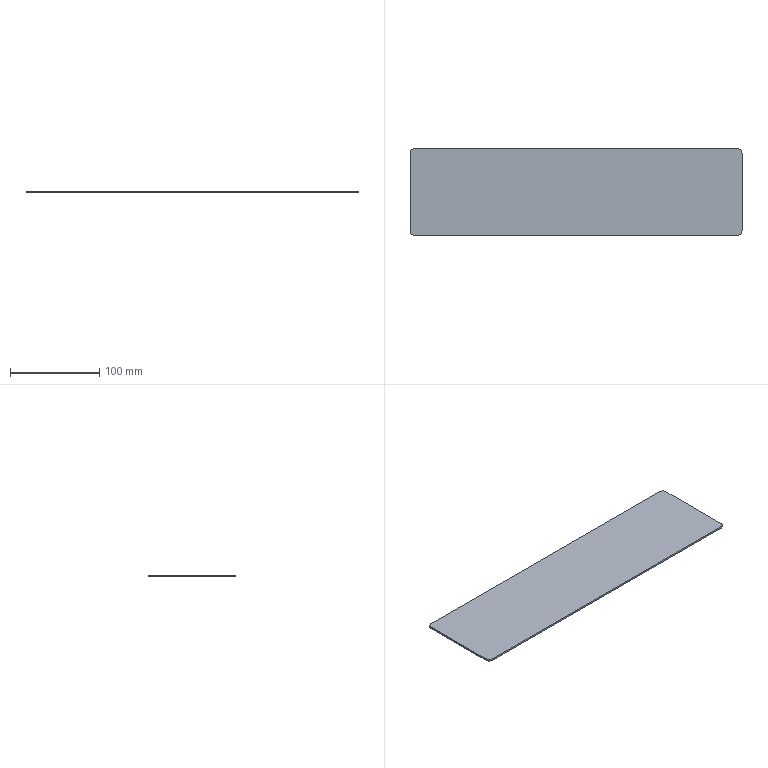Part | SolidWorks | features FlatPattern 1, SMBaseFlange 1, SheetMetal 1 | 1 solid | 10 faces | box 372 x 97 x 2 mm | volume 72125 mm3 | plane 6 | cylinder 4 | commonest cylinder face diameters 10 x4
STEP:
#1=CARTESIAN_POINT('',(0.,-92.,0.));
#2=VERTEX_POINT('',#1);
#3=CARTESIAN_POINT('',(5.,-97.,0.));
#4=VERTEX_POINT('',#3);
#5=CARTESIAN_POINT('',(5.,-92.,0.));
#6=DIRECTION('',(0.,0.,1.));
#7=DIRECTION('',(1.,0.,0.));
#8=AXIS2_PLACEMENT_3D('',#5,#6,#7);
#9=CIRCLE('',#8,5.);
#10=EDGE_CURVE('',#2,#4,#9,.T.);
#11=ORIENTED_EDGE('',*,*,#10,.F.);
#12=CARTESIAN_POINT('',(0.,-92.,-2.));
#13=VERTEX_POINT('',#12);
#14=CARTESIAN_POINT('',(0.,-92.,-2.));
#15=DIRECTION('',(0.,0.,1.));
#16=VECTOR('',#15,1000.);
#17=LINE('',#14,#16);
#18=EDGE_CURVE('',#13,#2,#17,.T.);
#19=ORIENTED_EDGE('',*,*,#18,.F.);
#20=CARTESIAN_POINT('',(5.,-97.,-2.));
#21=VERTEX_POINT('',#20);
#22=CARTESIAN_POINT('',(5.,-92.,-2.));
#23=DIRECTION('',(0.,0.,1.));
#24=DIRECTION('',(1.,0.,0.));
#25=AXIS2_PLACEMENT_3D('',#22,#23,#24);
#26=CIRCLE('',#25,5.);
#27=EDGE_CURVE('',#13,#21,#26,.T.);
#28=ORIENTED_EDGE('',*,*,#27,.T.);
#29=CARTESIAN_POINT('',(5.,-97.,-2.));
#30=DIRECTION('',(0.,0.,1.));
#31=VECTOR('',#30,1000.);
#32=LINE('',#29,#31);
#33=EDGE_CURVE('',#21,#4,#32,.T.);
#34=ORIENTED_EDGE('',*,*,#33,.T.);
#35=EDGE_LOOP('',(#11,#19,#28,#34));
#36=FACE_OUTER_BOUND('',#35,.T.);
#37=CARTESIAN_POINT('',(5.,-92.,-2.));
#38=DIRECTION('',(0.,0.,1.));
#39=DIRECTION('',(1.,0.,0.));
#40=AXIS2_PLACEMENT_3D('',#37,#38,#39);
#41=CYLINDRICAL_SURFACE('',#40,5.);
#42=ADVANCED_FACE('',(#36),#41,.T.);
#43=CARTESIAN_POINT('',(0.,-5.,0.));
#44=VERTEX_POINT('',#43);
#45=CARTESIAN_POINT('',(0.,-5.,0.));
#46=DIRECTION('',(0.,-1.,0.));
#47=VECTOR('',#46,1000.);
#48=LINE('',#45,#47);
#49=EDGE_CURVE('',#44,#2,#48,.T.);
#50=ORIENTED_EDGE('',*,*,#49,.F.);
#51=CARTESIAN_POINT('',(0.,-5.,-2.));
#52=VERTEX_POINT('',#51);
#53=CARTESIAN_POINT('',(0.,-5.,-2.));
#54=DIRECTION('',(0.,0.,1.));
#55=VECTOR('',#54,1000.);
#56=LINE('',#53,#55);
#57=EDGE_CURVE('',#52,#44,#56,.T.);
#58=ORIENTED_EDGE('',*,*,#57,.F.);
#59=CARTESIAN_POINT('',(0.,-5.,-2.));
#60=DIRECTION('',(0.,-1.,0.));
#61=VECTOR('',#60,1000.);
#62=LINE('',#59,#61);
#63=EDGE_CURVE('',#52,#13,#62,.T.);
#64=ORIENTED_EDGE('',*,*,#63,.T.);
#65=ORIENTED_EDGE('',*,*,#18,.T.);
#66=EDGE_LOOP('',(#50,#58,#64,#65));
#67=FACE_OUTER_BOUND('',#66,.T.);
#68=CARTESIAN_POINT('',(0.,-5.,-2.));
#69=DIRECTION('',(-1.,0.,0.));
#70=DIRECTION('',(0.,-1.,0.));
#71=AXIS2_PLACEMENT_3D('',#68,#69,#70);
#72=PLANE('',#71);
#73=ADVANCED_FACE('',(#67),#72,.T.);
#74=CARTESIAN_POINT('',(5.,0.,0.));
#75=VERTEX_POINT('',#74);
#76=CARTESIAN_POINT('',(5.,-5.,0.));
#77=DIRECTION('',(0.,0.,1.));
#78=DIRECTION('',(1.,0.,0.));
#79=AXIS2_PLACEMENT_3D('',#76,#77,#78);
#80=CIRCLE('',#79,5.);
#81=EDGE_CURVE('',#75,#44,#80,.T.);
#82=ORIENTED_EDGE('',*,*,#81,.F.);
#83=CARTESIAN_POINT('',(5.,0.,-2.));
#84=VERTEX_POINT('',#83);
#85=CARTESIAN_POINT('',(5.,0.,-2.));
#86=DIRECTION('',(0.,0.,1.));
#87=VECTOR('',#86,1000.);
#88=LINE('',#85,#87);
#89=EDGE_CURVE('',#84,#75,#88,.T.);
#90=ORIENTED_EDGE('',*,*,#89,.F.);
#91=CARTESIAN_POINT('',(5.,-5.,-2.));
#92=DIRECTION('',(0.,0.,1.));
#93=DIRECTION('',(1.,0.,0.));
#94=AXIS2_PLACEMENT_3D('',#91,#92,#93);
#95=CIRCLE('',#94,5.);
#96=EDGE_CURVE('',#84,#52,#95,.T.);
#97=ORIENTED_EDGE('',*,*,#96,.T.);
#98=ORIENTED_EDGE('',*,*,#57,.T.);
#99=EDGE_LOOP('',(#82,#90,#97,#98));
#100=FACE_OUTER_BOUND('',#99,.T.);
#101=CARTESIAN_POINT('',(5.,-5.,-2.));
#102=DIRECTION('',(0.,0.,1.));
#103=DIRECTION('',(1.,0.,0.));
#104=AXIS2_PLACEMENT_3D('',#101,#102,#103);
#105=CYLINDRICAL_SURFACE('',#104,5.);
#106=ADVANCED_FACE('',(#100),#105,.T.);
#107=CARTESIAN_POINT('',(367.,0.,0.));
#108=VERTEX_POINT('',#107);
#109=CARTESIAN_POINT('',(5.,0.,0.));
#110=DIRECTION('',(-1.,0.,0.));
#111=VECTOR('',#110,1000.);
#112=LINE('',#109,#111);
#113=EDGE_CURVE('',#108,#75,#112,.T.);
#114=ORIENTED_EDGE('',*,*,#113,.F.);
#115=CARTESIAN_POINT('',(367.,0.,-2.));
#116=VERTEX_POINT('',#115);
#117=CARTESIAN_POINT('',(367.,0.,-2.));
#118=DIRECTION('',(0.,0.,1.));
#119=VECTOR('',#118,1000.);
#120=LINE('',#117,#119);
#121=EDGE_CURVE('',#116,#108,#120,.T.);
#122=ORIENTED_EDGE('',*,*,#121,.F.);
#123=CARTESIAN_POINT('',(5.,0.,-2.));
#124=DIRECTION('',(-1.,0.,0.));
#125=VECTOR('',#124,1000.);
#126=LINE('',#123,#125);
#127=EDGE_CURVE('',#116,#84,#126,.T.);
#128=ORIENTED_EDGE('',*,*,#127,.T.);
#129=ORIENTED_EDGE('',*,*,#89,.T.);
#130=EDGE_LOOP('',(#114,#122,#128,#129));
#131=FACE_OUTER_BOUND('',#130,.T.);
#132=CARTESIAN_POINT('',(5.,0.,-2.));
#133=DIRECTION('',(0.,1.,0.));
#134=DIRECTION('',(0.,0.,1.));
#135=AXIS2_PLACEMENT_3D('',#132,#133,#134);
#136=PLANE('',#135);
#137=ADVANCED_FACE('',(#131),#136,.T.);
#138=CARTESIAN_POINT('',(372.,-5.,0.));
#139=VERTEX_POINT('',#138);
#140=CARTESIAN_POINT('',(367.,-5.,0.));
#141=DIRECTION('',(0.,0.,1.));
#142=DIRECTION('',(-1.,0.,0.));
#143=AXIS2_PLACEMENT_3D('',#140,#141,#142);
#144=CIRCLE('',#143,5.);
#145=EDGE_CURVE('',#139,#108,#144,.T.);
#146=ORIENTED_EDGE('',*,*,#145,.F.);
#147=CARTESIAN_POINT('',(372.,-5.,-2.));
#148=VERTEX_POINT('',#147);
#149=CARTESIAN_POINT('',(372.,-5.,-2.));
#150=DIRECTION('',(0.,0.,1.));
#151=VECTOR('',#150,1000.);
#152=LINE('',#149,#151);
#153=EDGE_CURVE('',#148,#139,#152,.T.);
#154=ORIENTED_EDGE('',*,*,#153,.F.);
#155=CARTESIAN_POINT('',(367.,-5.,-2.));
#156=DIRECTION('',(0.,0.,1.));
#157=DIRECTION('',(-1.,0.,0.));
#158=AXIS2_PLACEMENT_3D('',#155,#156,#157);
#159=CIRCLE('',#158,5.);
#160=EDGE_CURVE('',#148,#116,#159,.T.);
#161=ORIENTED_EDGE('',*,*,#160,.T.);
#162=ORIENTED_EDGE('',*,*,#121,.T.);
#163=EDGE_LOOP('',(#146,#154,#161,#162));
#164=FACE_OUTER_BOUND('',#163,.T.);
#165=CARTESIAN_POINT('',(367.,-5.,-2.));
#166=DIRECTION('',(0.,0.,1.));
#167=DIRECTION('',(1.,0.,0.));
#168=AXIS2_PLACEMENT_3D('',#165,#166,#167);
#169=CYLINDRICAL_SURFACE('',#168,5.);
#170=ADVANCED_FACE('',(#164),#169,.T.);
#171=CARTESIAN_POINT('',(372.,-92.,0.));
#172=VERTEX_POINT('',#171);
#173=CARTESIAN_POINT('',(372.,-5.,0.));
#174=DIRECTION('',(0.,1.,0.));
#175=VECTOR('',#174,1000.);
#176=LINE('',#173,#175);
#177=EDGE_CURVE('',#172,#139,#176,.T.);
#178=ORIENTED_EDGE('',*,*,#177,.F.);
#179=CARTESIAN_POINT('',(372.,-92.,-2.));
#180=VERTEX_POINT('',#179);
#181=CARTESIAN_POINT('',(372.,-92.,-2.));
#182=DIRECTION('',(0.,0.,1.));
#183=VECTOR('',#182,1000.);
#184=LINE('',#181,#183);
#185=EDGE_CURVE('',#180,#172,#184,.T.);
#186=ORIENTED_EDGE('',*,*,#185,.F.);
#187=CARTESIAN_POINT('',(372.,-5.,-2.));
#188=DIRECTION('',(0.,1.,0.));
#189=VECTOR('',#188,1000.);
#190=LINE('',#187,#189);
#191=EDGE_CURVE('',#180,#148,#190,.T.);
#192=ORIENTED_EDGE('',*,*,#191,.T.);
#193=ORIENTED_EDGE('',*,*,#153,.T.);
#194=EDGE_LOOP('',(#178,#186,#192,#193));
#195=FACE_OUTER_BOUND('',#194,.T.);
#196=CARTESIAN_POINT('',(372.,-5.,-2.));
#197=DIRECTION('',(1.,0.,0.));
#198=DIRECTION('',(0.,0.,-1.));
#199=AXIS2_PLACEMENT_3D('',#196,#197,#198);
#200=PLANE('',#199);
#201=ADVANCED_FACE('',(#195),#200,.T.);
#202=CARTESIAN_POINT('',(367.,-97.,0.));
#203=VERTEX_POINT('',#202);
#204=CARTESIAN_POINT('',(367.,-92.,0.));
#205=DIRECTION('',(0.,0.,1.));
#206=DIRECTION('',(1.,0.,0.));
#207=AXIS2_PLACEMENT_3D('',#204,#205,#206);
#208=CIRCLE('',#207,5.);
#209=EDGE_CURVE('',#203,#172,#208,.T.);
#210=ORIENTED_EDGE('',*,*,#209,.F.);
#211=CARTESIAN_POINT('',(367.,-97.,-2.));
#212=VERTEX_POINT('',#211);
#213=CARTESIAN_POINT('',(367.,-97.,-2.));
#214=DIRECTION('',(0.,0.,1.));
#215=VECTOR('',#214,1000.);
#216=LINE('',#213,#215);
#217=EDGE_CURVE('',#212,#203,#216,.T.);
#218=ORIENTED_EDGE('',*,*,#217,.F.);
#219=CARTESIAN_POINT('',(367.,-92.,-2.));
#220=DIRECTION('',(0.,0.,1.));
#221=DIRECTION('',(1.,0.,0.));
#222=AXIS2_PLACEMENT_3D('',#219,#220,#221);
#223=CIRCLE('',#222,5.);
#224=EDGE_CURVE('',#212,#180,#223,.T.);
#225=ORIENTED_EDGE('',*,*,#224,.T.);
#226=ORIENTED_EDGE('',*,*,#185,.T.);
#227=EDGE_LOOP('',(#210,#218,#225,#226));
#228=FACE_OUTER_BOUND('',#227,.T.);
#229=CARTESIAN_POINT('',(367.,-92.,-2.));
#230=DIRECTION('',(0.,0.,1.));
#231=DIRECTION('',(1.,0.,0.));
#232=AXIS2_PLACEMENT_3D('',#229,#230,#231);
#233=CYLINDRICAL_SURFACE('',#232,5.);
#234=ADVANCED_FACE('',(#228),#233,.T.);
#235=CARTESIAN_POINT('',(5.,-97.,0.));
#236=DIRECTION('',(1.,0.,0.));
#237=VECTOR('',#236,1000.);
#238=LINE('',#235,#237);
#239=EDGE_CURVE('',#4,#203,#238,.T.);
#240=ORIENTED_EDGE('',*,*,#239,.F.);
#241=ORIENTED_EDGE('',*,*,#33,.F.);
#242=CARTESIAN_POINT('',(5.,-97.,-2.));
#243=DIRECTION('',(1.,0.,0.));
#244=VECTOR('',#243,1000.);
#245=LINE('',#242,#244);
#246=EDGE_CURVE('',#21,#212,#245,.T.);
#247=ORIENTED_EDGE('',*,*,#246,.T.);
#248=ORIENTED_EDGE('',*,*,#217,.T.);
#249=EDGE_LOOP('',(#240,#241,#247,#248));
#250=FACE_OUTER_BOUND('',#249,.T.);
#251=CARTESIAN_POINT('',(5.,-97.,-2.));
#252=DIRECTION('',(0.,-1.,0.));
#253=DIRECTION('',(0.,0.,-1.));
#254=AXIS2_PLACEMENT_3D('',#251,#252,#253);
#255=PLANE('',#254);
#256=ADVANCED_FACE('',(#250),#255,.T.);
#257=ORIENTED_EDGE('',*,*,#27,.F.);
#258=ORIENTED_EDGE('',*,*,#63,.F.);
#259=ORIENTED_EDGE('',*,*,#96,.F.);
#260=ORIENTED_EDGE('',*,*,#127,.F.);
#261=ORIENTED_EDGE('',*,*,#160,.F.);
#262=ORIENTED_EDGE('',*,*,#191,.F.);
#263=ORIENTED_EDGE('',*,*,#224,.F.);
#264=ORIENTED_EDGE('',*,*,#246,.F.);
#265=EDGE_LOOP('',(#257,#258,#259,#260,#261,#262,#263,#264));
#266=FACE_OUTER_BOUND('',#265,.T.);
#267=CARTESIAN_POINT('',(5.,-92.,-2.));
#268=DIRECTION('',(0.,0.,1.));
#269=DIRECTION('',(1.,0.,0.));
#270=AXIS2_PLACEMENT_3D('',#267,#268,#269);
#271=PLANE('',#270);
#272=ADVANCED_FACE('',(#266),#271,.F.);
#273=ORIENTED_EDGE('',*,*,#10,.T.);
#274=ORIENTED_EDGE('',*,*,#239,.T.);
#275=ORIENTED_EDGE('',*,*,#209,.T.);
#276=ORIENTED_EDGE('',*,*,#177,.T.);
#277=ORIENTED_EDGE('',*,*,#145,.T.);
#278=ORIENTED_EDGE('',*,*,#113,.T.);
#279=ORIENTED_EDGE('',*,*,#81,.T.);
#280=ORIENTED_EDGE('',*,*,#49,.T.);
#281=EDGE_LOOP('',(#273,#274,#275,#276,#277,#278,#279,#280));
#282=FACE_OUTER_BOUND('',#281,.T.);
#283=CARTESIAN_POINT('',(5.,-92.,0.));
#284=DIRECTION('',(0.,0.,1.));
#285=DIRECTION('',(1.,0.,0.));
#286=AXIS2_PLACEMENT_3D('',#283,#284,#285);
#287=PLANE('',#286);
#288=ADVANCED_FACE('',(#282),#287,.T.);
#289=CLOSED_SHELL('',(#42,#73,#106,#137,#170,#201,#234,#256,#272,#288));
#290=MANIFOLD_SOLID_BREP('',#289);
#291=CARTESIAN_POINT('',(0.,0.,0.));
#292=DIRECTION('',(0.,0.,1.));
#293=DIRECTION('',(1.,0.,0.));
#294=AXIS2_PLACEMENT_3D('',#291,#292,#293);
#295=(LENGTH_UNIT()NAMED_UNIT(*)SI_UNIT(.MILLI.,.METRE.));
#296=UNCERTAINTY_MEASURE_WITH_UNIT(LENGTH_MEASURE(0.00001),#295,'','');
#297=(NAMED_UNIT(*)PLANE_ANGLE_UNIT()SI_UNIT($,.RADIAN.));
#298=(NAMED_UNIT(*)SI_UNIT($,.STERADIAN.)SOLID_ANGLE_UNIT());
#299=(GEOMETRIC_REPRESENTATION_CONTEXT(3)GLOBAL_UNCERTAINTY_ASSIGNED_CONTEXT((#296))GLOBAL_UNIT_ASSIGNED_CONTEXT((#295,#297,#298))REPRESENTATION_CONTEXT('',''));
#300=ADVANCED_BREP_SHAPE_REPRESENTATION('',(#290,#294),#299);